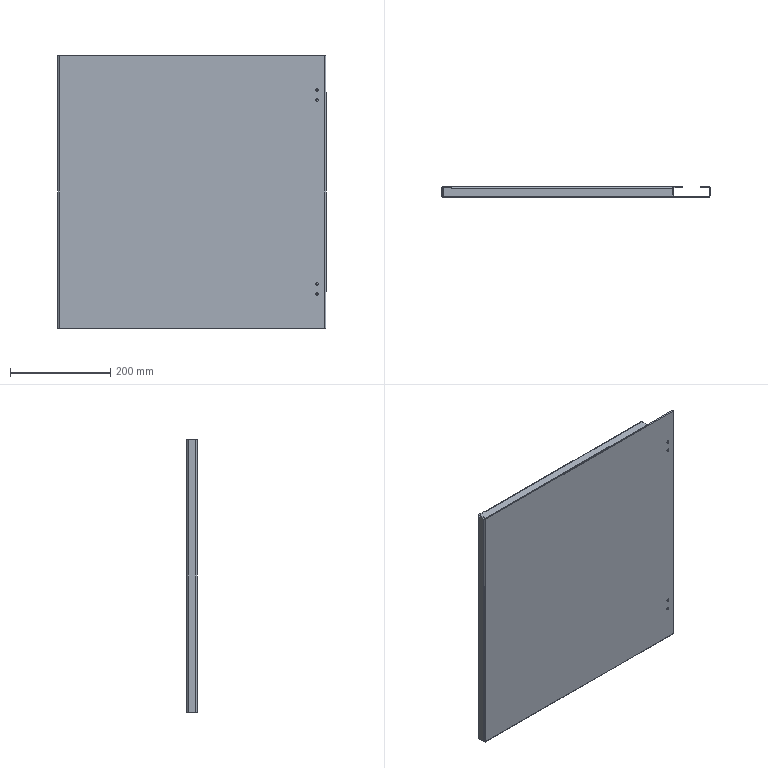Part | NX | features BREP 1 | 1 solid | 74 faces | box 534.5 x 20 x 546 mm | volume 536019 mm3 | plane 52 | cylinder 22 | commonest cylinder face diameters 3 x8 5 x8 6 x6